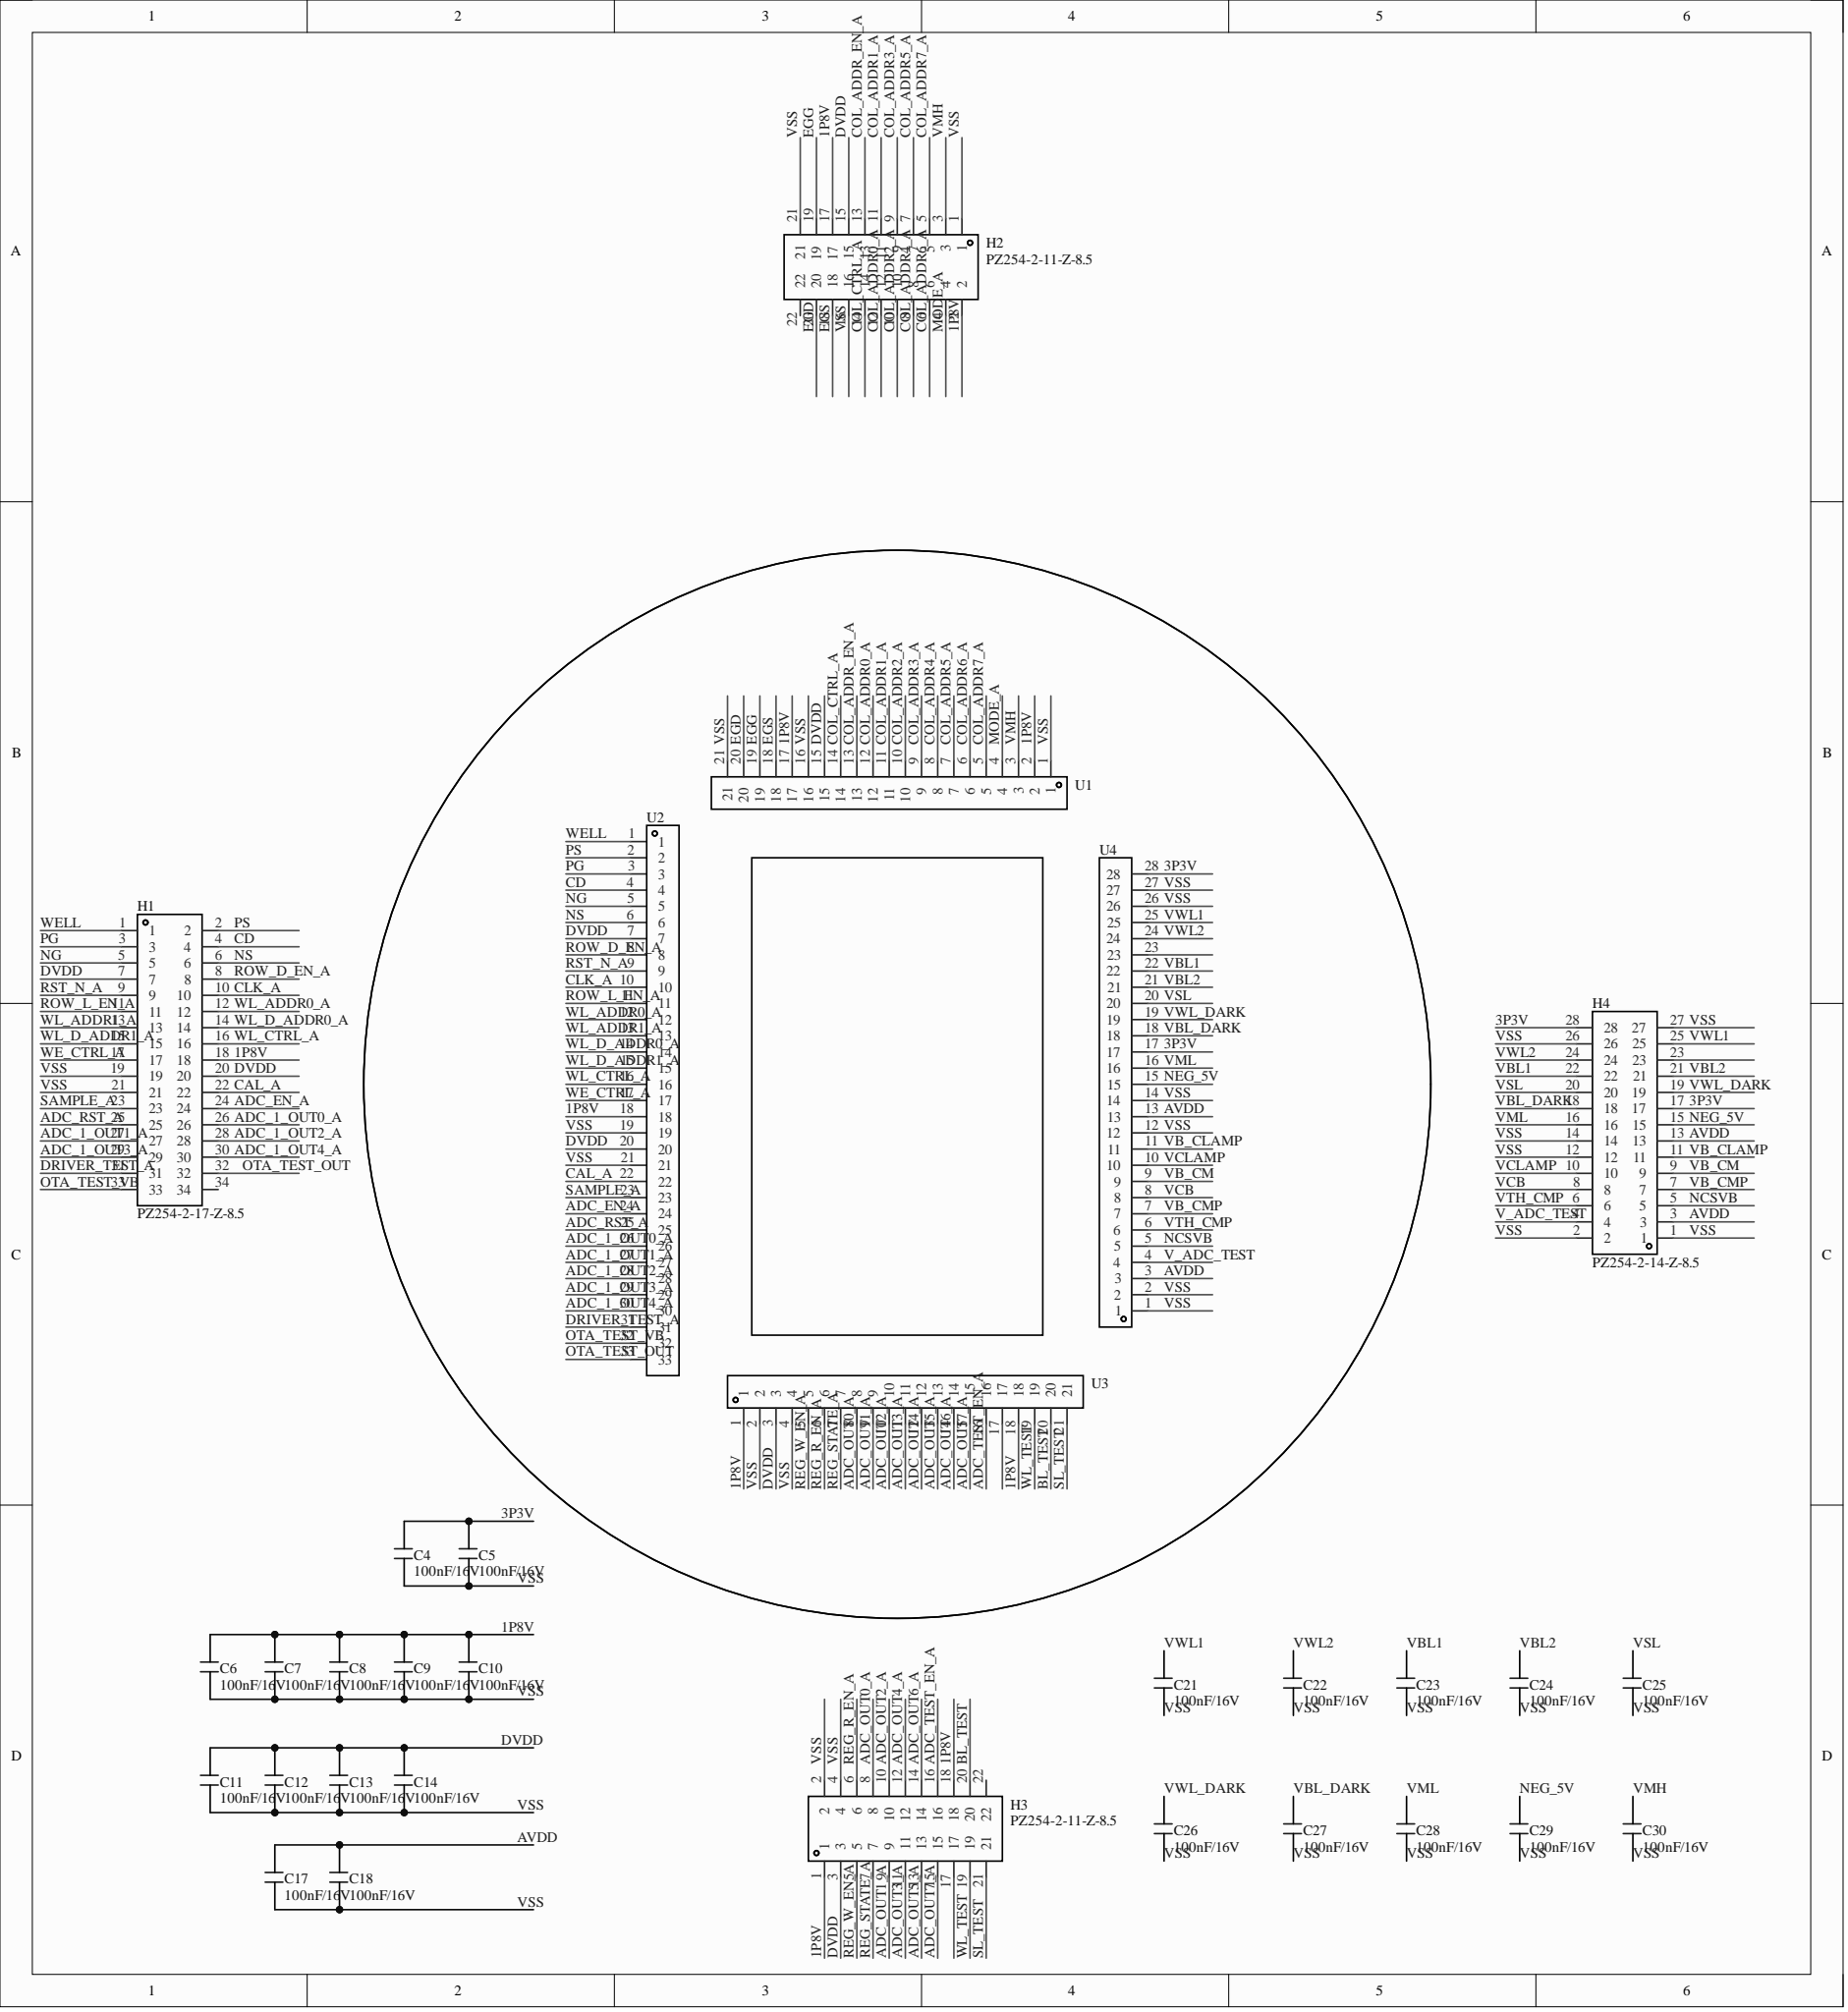Circuit board | Altium Designer | 31 parts | 80 nets
Bill of materials:
Comment,Description,Designator,Footprint,LibRef,Quantity
"100nF/16V","component CAP componentdescr capacitor model","C4, C5, C6, C7, C8, C9, C10, C11, C12, C13, C14, C17, C18, C21, C22, C23, C24, C25, C26, C27, C28, C29, C30","0603C","CAP","23"
"PZ254-2-17-Z-8.5","","H1","HDR-TH_34P-P2.54-V-M-R2-C17-S2.54","PZ254-2-17-Z-8.5","1"
"PZ254-2-11-Z-8.5","","H2, H3","HDR-TH_22P-P2.54-V-M-R2-C11-S2.54","PZ254-2-11-Z-8.5","2"
"PZ254-2-14-Z-8.5","","H4","HDR-TH_28P-P2.54-V-M-R2-C14-S2.54","PZ254-2-14-Z-8.5","1"
"X6511WVS-21H-C60D48R2","","U1, U3","JSZ21","X6511WVS-21H-C60D48R2","2"
"X6511WVS-33H-C60D48R2","","U2","JSZ33","X6511WVS-33H-C60D48R2","1"
"X6511WVS-28H-C60D48R1","","U4","JSZ28","X6511WVS-28H-C60D48R1","1"
Netlist (Protel format):
[
C4
0603C
100nF/16V



]
[
C5
0603C
100nF/16V



]
[
C6
0603C
100nF/16V



]
[
C7
0603C
100nF/16V



]
[
C8
0603C
100nF/16V



]
[
C9
0603C
100nF/16V



]
[
C10
0603C
100nF/16V



]
[
C11
0603C
100nF/16V



]
[
C12
0603C
100nF/16V



]
[
C13
0603C
100nF/16V



]
[
C14
0603C
100nF/16V



]
[
C17
0603C
100nF/16V



]
[
C18
0603C
100nF/16V



]
[
C21
0603C
100nF/16V



]
[
C22
0603C
100nF/16V



]
[
C23
0603C
100nF/16V



]
[
C24
0603C
100nF/16V



]
[
C25
0603C
100nF/16V



]
[
C26
0603C
100nF/16V



]
[
C27
0603C
100nF/16V



]
[
C28
0603C
100nF/16V



]
[
C29
0603C
100nF/16V



]
[
C30
0603C
100nF/16V



]
[
H1
HDR-TH_34P-P2.54-V-M-R2-C17-S2.54
PZ254-2-17-Z-8.5



]
[
H2
HDR-TH_22P-P2.54-V-M-R2-C11-S2.54
PZ254-2-11-Z-8.5



]
[
H3
HDR-TH_22P-P2.54-V-M-R2-C11-S2.54
PZ254-2-11-Z-8.5



]
[
H4
HDR-TH_28P-P2.54-V-M-R2-C14-S2.54
PZ254-2-14-Z-8.5



]
[
U1
JSZ21
X6511WVS-21H-C60D48R2



]
[
U2
JSZ33
X6511WVS-33H-C60D48R2



]
[
U3
JSZ21
X6511WVS-21H-C60D48R2



]
[
U4
JSZ28
X6511WVS-28H-C60D48R1



]
(
WL_TEST
H3-19
U3-19
)
(
WL_D_ADDR1_A
H1-15
U2-15
)
(
WL_D_ADDR0_A
H1-14
U2-14
)
(
WL_CTRL_A
H1-16
U2-16
)
(
WL_ADDR1_A
H1-13
U2-13
)
(
WL_ADDR0_A
H1-12
U2-12
)
(
WELL
H1-1
U2-1
)
(
WE_CTRL_A
H1-17
U2-17
)
(
VWL_DARK
C26-1
H4-19
U4-19
)
(
VWL2
C22-1
H4-24
U4-24
)
(
VWL1
C21-1
H4-25
U4-25
)
(
VTH_CMP
H4-6
U4-6
)
(
VSS
C4-2
C5-2
C6-2
C7-2
C8-2
C9-2
C10-2
C11-2
C12-2
C13-2
C14-2
C17-2
C18-2
C21-2
C22-2
C23-2
C24-2
C25-2
C26-2
C27-2
C28-2
C29-2
C30-2
H1-19
H1-21
H2-1
H2-16
H2-21
H3-2
H3-4
H4-1
H4-2
H4-12
H4-14
H4-26
H4-27
U1-1
U1-16
U1-21
U2-19
U2-21
U3-2
U3-4
U4-1
U4-2
U4-12
U4-14
U4-26
U4-27
)
(
VSL
C25-1
H4-20
U4-20
)
(
VML
C28-1
H4-16
U4-16
)
(
VMH
C30-1
H2-3
U1-3
)
(
VCLAMP
H4-10
U4-10
)
(
VCB
H4-8
U4-8
)
(
VBL_DARK
C27-1
H4-18
U4-18
)
(
VBL2
C24-1
H4-21
U4-21
)
(
VBL1
C23-1
H4-22
U4-22
)
(
VB_CMP
H4-7
U4-7
)
(
VB_CM
H4-9
U4-9
)
(
VB_CLAMP
H4-11
U4-11
)
(
V_ADC_TEST
H4-4
U4-4
)
(
SL_TEST
H3-21
U3-21
)
(
SAMPLE_A
H1-23
U2-23
)
(
RST_N_A
H1-9
U2-9
)
(
ROW_L_EN_A
H1-11
U2-11
)
(
ROW_D_EN_A
H1-8
U2-8
)
(
REG_W_EN_A
H3-5
U3-5
)
(
REG_STATE_A
H3-7
U3-7
)
(
REG_R_EN_A
H3-6
U3-6
)
(
PS
H1-2
U2-2
)
(
PG
H1-3
U2-3
)
(
OTA_TEST_VB
H1-33
U2-32
)
(
OTA_TEST_OUT
H1-32
U2-33
)
(
NS
H1-6
U2-6
)
(
NG
H1-5
U2-5
)
(
NEG_5V
C29-1
H4-15
U4-15
)
(
NCSVB
H4-5
U4-5
)
(
MODE_A
H2-4
U1-4
)
(
EGS
H2-18
U1-18
)
(
EGG
H2-19
U1-19
)
(
EGD
H2-20
U1-20
)
(
DVDD
C11-1
C12-1
C13-1
C14-1
H1-7
H1-20
H2-15
H3-3
U1-15
U2-7
U2-20
U3-3
)
(
DRIVER_TEST_A
H1-31
U2-31
)
(
COL_CTRL_A
H2-14
U1-14
)
(
COL_ADDR_EN_A
H2-13
U1-13
)
(
COL_ADDR7_A
H2-5
U1-5
)
(
COL_ADDR6_A
H2-6
U1-6
)
(
COL_ADDR5_A
H2-7
U1-7
)
(
COL_ADDR4_A
H2-8
U1-8
)
(
COL_ADDR3_A
H2-9
U1-9
)
(
COL_ADDR2_A
H2-10
U1-10
)
(
COL_ADDR1_A
H2-11
U1-11
)
(
COL_ADDR0_A
H2-12
U1-12
)
(
CLK_A
H1-10
U2-10
)
(
CD
H1-4
U2-4
)
(
CAL_A
H1-22
U2-22
)
(
BL_TEST
H3-20
U3-20
)
(
AVDD
C17-1
C18-1
H4-3
H4-13
U4-3
U4-13
)
(
ADC_TEST_EN_A
H3-16
U3-16
)
(
ADC_RST_A
H1-25
U2-25
)
(
ADC_OUT7_A
H3-15
U3-15
)
(
ADC_OUT6_A
H3-14
U3-14
)
(
ADC_OUT5_A
H3-13
U3-13
)
(
ADC_OUT4_A
H3-12
U3-12
)
(
ADC_OUT3_A
H3-11
U3-11
)
(
ADC_OUT2_A
H3-10
U3-10
)
(
ADC_OUT1_A
H3-9
U3-9
)
(
ADC_OUT0_A
H3-8
U3-8
)
(
ADC_EN_A
H1-24
U2-24
)
(
ADC_1_OUT4_A
H1-30
U2-30
)
(
ADC_1_OUT3_A
H1-29
U2-29
)
(
ADC_1_OUT2_A
H1-28
U2-28
)
(
ADC_1_OUT1_A
H1-27
U2-27
)
(
ADC_1_OUT0_A
H1-26
U2-26
)
(
3P3V
C4-1
C5-1
H4-17
H4-28
U4-17
U4-28
)
(
1P8V
C6-1
C7-1
C8-1
C9-1
C10-1
H1-18
H2-2
H2-17
H3-1
H3-18
U1-2
U1-17
U2-18
U3-1
U3-18
)